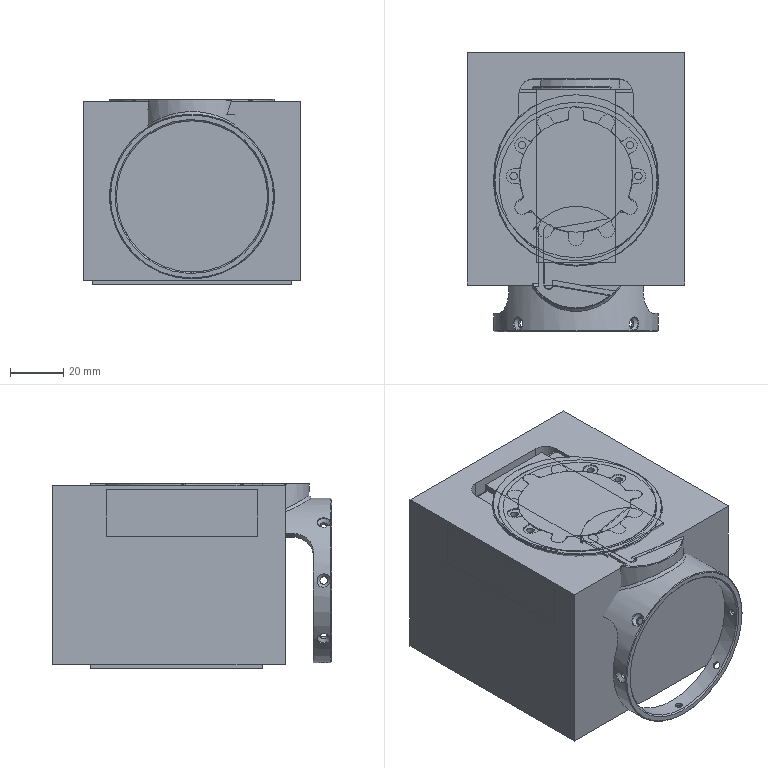Part | 6 solids | 642 faces | box 82 x 105.2 x 70 mm | volume 778596 mm3 | cylinder 279 | plane 258 | cone 71 | spline 34 | commonest cylinder face diameters 2 x66 2.8 x48 5.5 x39 5 x21 4 x18 1.6 x12